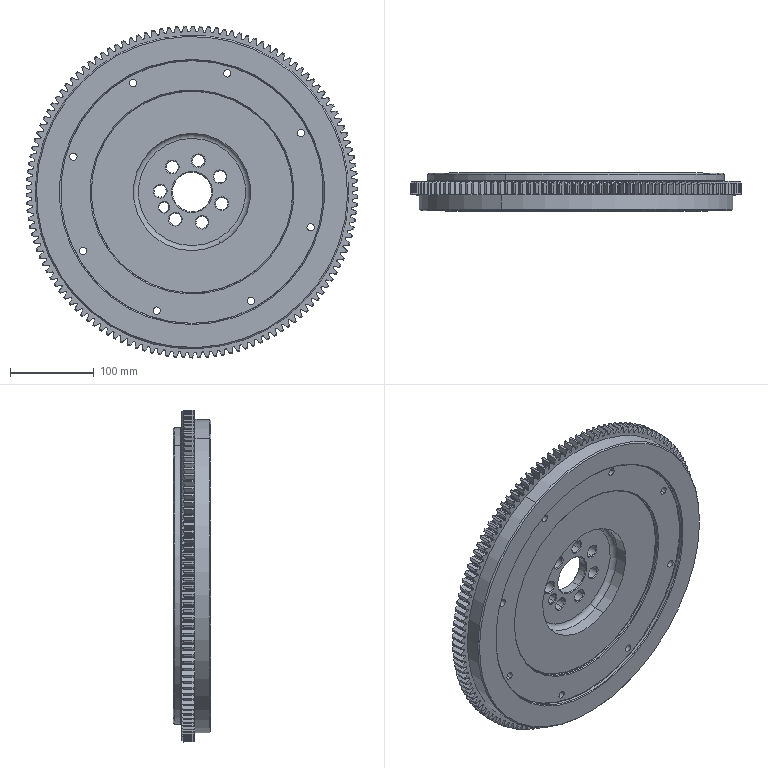Part | SolidWorks | features BaseBody 2 | 2 solids | 1595 faces | box 395.969 x 45 x 396 mm | volume 3364206 mm3 | plane 674 | cylinder 599 | cone 312 | torus 10 | commonest cylinder face diameters 2 x260 396 x131 382.5 x130 6.985 x16 8.782 x16 14.5 x14